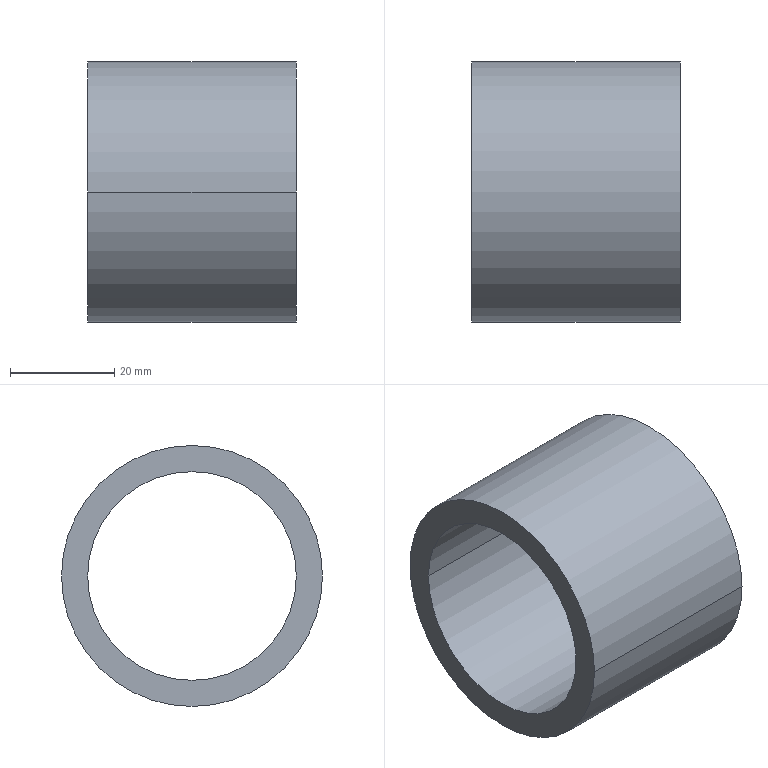Part | STEP file | P-0082107 | 1 solid | 6 faces | box 40 x 50 x 50 mm | volume 28274 mm3 | cylinder 4 | plane 2 | commonest cylinder face diameters 40 x2 50 x2
STEP:
#1=CARTESIAN_POINT('',(0.,0.,0.));
#2=DIRECTION('',(0.,0.,1.));
#3=DIRECTION('',(1.,0.,0.));
#4=AXIS2_PLACEMENT_3D('',#1,#2,#3);
#5=CARTESIAN_POINT('',(-30.,20.,0.));
#6=VERTEX_POINT('',#5);
#7=CARTESIAN_POINT('',(-30.,-20.,0.));
#8=VERTEX_POINT('',#7);
#9=CARTESIAN_POINT('',(-30.,0.,0.));
#10=DIRECTION('',(-1.,0.,0.));
#11=DIRECTION('',(0.,1.,0.));
#12=AXIS2_PLACEMENT_3D('',#9,#10,#11);
#13=CIRCLE('',#12,20.);
#14=CARTESIAN_POINT('',(-30.,0.,0.));
#15=DIRECTION('',(1.,0.,0.));
#16=DIRECTION('',(0.,1.,0.));
#17=AXIS2_PLACEMENT_3D('',#14,#15,#16);
#18=PLANE('',#17);
#19=CARTESIAN_POINT('',(20.,0.));
#20=CARTESIAN_POINT('',(20.,-34.641));
#21=CARTESIAN_POINT('',(-10.,-17.321));
#22=CARTESIAN_POINT('',(-40.,0.));
#23=CARTESIAN_POINT('',(-10.,17.321));
#24=CARTESIAN_POINT('',(20.,34.641));
#25=CARTESIAN_POINT('',(20.,0.));
#26=(BOUNDED_CURVE()B_SPLINE_CURVE(2,(#19,#20,#21,#22,#23,#24,#25),.UNSPECIFIED.,.T.,.F.)B_SPLINE_CURVE_WITH_KNOTS((1,2,2,2,2,1),(-2.094,0.,2.094,4.189,6.283,8.378),.UNSPECIFIED.)CURVE()GEOMETRIC_REPRESENTATION_ITEM()RATIONAL_B_SPLINE_CURVE((1.,0.5,1.,0.5,1.,0.5,1.))REPRESENTATION_ITEM(''));
#27=(GEOMETRIC_REPRESENTATION_CONTEXT(2)PARAMETRIC_REPRESENTATION_CONTEXT()REPRESENTATION_CONTEXT('',''));
#28=DEFINITIONAL_REPRESENTATION('',(#26),#27);
#29=PCURVE('',#18,#28);
#30=CARTESIAN_POINT('',(-30.,0.,0.));
#31=DIRECTION('',(1.,0.,0.));
#32=DIRECTION('',(0.,1.,0.));
#33=AXIS2_PLACEMENT_3D('',#30,#31,#32);
#34=CYLINDRICAL_SURFACE('',#33,20.);
#35=CARTESIAN_POINT('',(6.283,0.));
#36=DIRECTION('',(-1.,0.));
#37=VECTOR('',#36,1.);
#38=LINE('',#35,#37);
#39=(GEOMETRIC_REPRESENTATION_CONTEXT(2)PARAMETRIC_REPRESENTATION_CONTEXT()REPRESENTATION_CONTEXT('',''));
#40=DEFINITIONAL_REPRESENTATION('',(#38),#39);
#41=PCURVE('',#34,#40);
#42=SURFACE_CURVE('',#13,(#29,#41),.PCURVE_S1.);
#43=EDGE_CURVE('',#6,#8,#42,.T.);
#44=ORIENTED_EDGE('',*,*,#43,.F.);
#45=CARTESIAN_POINT('',(-30.,0.,0.));
#46=DIRECTION('',(-1.,0.,0.));
#47=DIRECTION('',(0.,1.,0.));
#48=AXIS2_PLACEMENT_3D('',#45,#46,#47);
#49=CIRCLE('',#48,20.);
#50=CARTESIAN_POINT('',(20.,0.));
#51=CARTESIAN_POINT('',(20.,-34.641));
#52=CARTESIAN_POINT('',(-10.,-17.321));
#53=CARTESIAN_POINT('',(-40.,0.));
#54=CARTESIAN_POINT('',(-10.,17.321));
#55=CARTESIAN_POINT('',(20.,34.641));
#56=CARTESIAN_POINT('',(20.,0.));
#57=(BOUNDED_CURVE()B_SPLINE_CURVE(2,(#50,#51,#52,#53,#54,#55,#56),.UNSPECIFIED.,.T.,.F.)B_SPLINE_CURVE_WITH_KNOTS((1,2,2,2,2,1),(-2.094,0.,2.094,4.189,6.283,8.378),.UNSPECIFIED.)CURVE()GEOMETRIC_REPRESENTATION_ITEM()RATIONAL_B_SPLINE_CURVE((1.,0.5,1.,0.5,1.,0.5,1.))REPRESENTATION_ITEM(''));
#58=(GEOMETRIC_REPRESENTATION_CONTEXT(2)PARAMETRIC_REPRESENTATION_CONTEXT()REPRESENTATION_CONTEXT('',''));
#59=DEFINITIONAL_REPRESENTATION('',(#57),#58);
#60=PCURVE('',#18,#59);
#61=CARTESIAN_POINT('',(-30.,0.,0.));
#62=DIRECTION('',(1.,0.,0.));
#63=DIRECTION('',(0.,1.,0.));
#64=AXIS2_PLACEMENT_3D('',#61,#62,#63);
#65=CYLINDRICAL_SURFACE('',#64,20.);
#66=CARTESIAN_POINT('',(6.283,0.));
#67=DIRECTION('',(-1.,0.));
#68=VECTOR('',#67,1.);
#69=LINE('',#66,#68);
#70=(GEOMETRIC_REPRESENTATION_CONTEXT(2)PARAMETRIC_REPRESENTATION_CONTEXT()REPRESENTATION_CONTEXT('',''));
#71=DEFINITIONAL_REPRESENTATION('',(#69),#70);
#72=PCURVE('',#65,#71);
#73=SURFACE_CURVE('',#49,(#60,#72),.PCURVE_S1.);
#74=EDGE_CURVE('',#8,#6,#73,.T.);
#75=ORIENTED_EDGE('',*,*,#74,.F.);
#76=EDGE_LOOP('',(#44,#75));
#77=FACE_BOUND('',#76,.T.);
#78=CARTESIAN_POINT('',(-30.,25.,0.));
#79=VERTEX_POINT('',#78);
#80=CARTESIAN_POINT('',(-30.,-25.,0.));
#81=VERTEX_POINT('',#80);
#82=CARTESIAN_POINT('',(-30.,0.,0.));
#83=DIRECTION('',(1.,0.,0.));
#84=DIRECTION('',(0.,1.,0.));
#85=AXIS2_PLACEMENT_3D('',#82,#83,#84);
#86=CIRCLE('',#85,25.);
#87=CARTESIAN_POINT('',(0.,0.));
#88=DIRECTION('',(1.,0.));
#89=AXIS2_PLACEMENT_2D('',#87,#88);
#90=CIRCLE('',#89,25.);
#91=(GEOMETRIC_REPRESENTATION_CONTEXT(2)PARAMETRIC_REPRESENTATION_CONTEXT()REPRESENTATION_CONTEXT('',''));
#92=DEFINITIONAL_REPRESENTATION('',(#90),#91);
#93=PCURVE('',#18,#92);
#94=CARTESIAN_POINT('',(-30.,0.,0.));
#95=DIRECTION('',(1.,0.,0.));
#96=DIRECTION('',(0.,1.,0.));
#97=AXIS2_PLACEMENT_3D('',#94,#95,#96);
#98=CYLINDRICAL_SURFACE('',#97,25.);
#99=CARTESIAN_POINT('',(0.,0.));
#100=DIRECTION('',(1.,0.));
#101=VECTOR('',#100,1.);
#102=LINE('',#99,#101);
#103=(GEOMETRIC_REPRESENTATION_CONTEXT(2)PARAMETRIC_REPRESENTATION_CONTEXT()REPRESENTATION_CONTEXT('',''));
#104=DEFINITIONAL_REPRESENTATION('',(#102),#103);
#105=PCURVE('',#98,#104);
#106=SURFACE_CURVE('',#86,(#93,#105),.PCURVE_S1.);
#107=EDGE_CURVE('',#79,#81,#106,.T.);
#108=ORIENTED_EDGE('',*,*,#107,.F.);
#109=CARTESIAN_POINT('',(-30.,0.,0.));
#110=DIRECTION('',(1.,0.,0.));
#111=DIRECTION('',(0.,1.,0.));
#112=AXIS2_PLACEMENT_3D('',#109,#110,#111);
#113=CIRCLE('',#112,25.);
#114=CARTESIAN_POINT('',(0.,0.));
#115=DIRECTION('',(1.,0.));
#116=AXIS2_PLACEMENT_2D('',#114,#115);
#117=CIRCLE('',#116,25.);
#118=(GEOMETRIC_REPRESENTATION_CONTEXT(2)PARAMETRIC_REPRESENTATION_CONTEXT()REPRESENTATION_CONTEXT('',''));
#119=DEFINITIONAL_REPRESENTATION('',(#117),#118);
#120=PCURVE('',#18,#119);
#121=CARTESIAN_POINT('',(-30.,0.,0.));
#122=DIRECTION('',(1.,0.,0.));
#123=DIRECTION('',(0.,1.,0.));
#124=AXIS2_PLACEMENT_3D('',#121,#122,#123);
#125=CYLINDRICAL_SURFACE('',#124,25.);
#126=CARTESIAN_POINT('',(0.,0.));
#127=DIRECTION('',(1.,0.));
#128=VECTOR('',#127,1.);
#129=LINE('',#126,#128);
#130=(GEOMETRIC_REPRESENTATION_CONTEXT(2)PARAMETRIC_REPRESENTATION_CONTEXT()REPRESENTATION_CONTEXT('',''));
#131=DEFINITIONAL_REPRESENTATION('',(#129),#130);
#132=PCURVE('',#125,#131);
#133=SURFACE_CURVE('',#113,(#120,#132),.PCURVE_S1.);
#134=EDGE_CURVE('',#81,#79,#133,.T.);
#135=ORIENTED_EDGE('',*,*,#134,.F.);
#136=EDGE_LOOP('',(#108,#135));
#137=FACE_BOUND('',#136,.T.);
#138=ADVANCED_FACE('',(#77,#137),#18,.F.);
#139=CARTESIAN_POINT('',(10.,20.,0.));
#140=VERTEX_POINT('',#139);
#141=CARTESIAN_POINT('',(10.,-20.,0.));
#142=VERTEX_POINT('',#141);
#143=CARTESIAN_POINT('',(10.,0.,0.));
#144=DIRECTION('',(1.,0.,0.));
#145=DIRECTION('',(0.,1.,0.));
#146=AXIS2_PLACEMENT_3D('',#143,#144,#145);
#147=CIRCLE('',#146,20.);
#148=CARTESIAN_POINT('',(10.,0.,0.));
#149=DIRECTION('',(1.,0.,0.));
#150=DIRECTION('',(0.,1.,0.));
#151=AXIS2_PLACEMENT_3D('',#148,#149,#150);
#152=PLANE('',#151);
#153=CARTESIAN_POINT('',(0.,0.));
#154=DIRECTION('',(1.,0.));
#155=AXIS2_PLACEMENT_2D('',#153,#154);
#156=CIRCLE('',#155,20.);
#157=(GEOMETRIC_REPRESENTATION_CONTEXT(2)PARAMETRIC_REPRESENTATION_CONTEXT()REPRESENTATION_CONTEXT('',''));
#158=DEFINITIONAL_REPRESENTATION('',(#156),#157);
#159=PCURVE('',#152,#158);
#160=CARTESIAN_POINT('',(0.,40.));
#161=DIRECTION('',(1.,0.));
#162=VECTOR('',#161,1.);
#163=LINE('',#160,#162);
#164=(GEOMETRIC_REPRESENTATION_CONTEXT(2)PARAMETRIC_REPRESENTATION_CONTEXT()REPRESENTATION_CONTEXT('',''));
#165=DEFINITIONAL_REPRESENTATION('',(#163),#164);
#166=PCURVE('',#65,#165);
#167=SURFACE_CURVE('',#147,(#159,#166),.PCURVE_S1.);
#168=EDGE_CURVE('',#140,#142,#167,.T.);
#169=ORIENTED_EDGE('',*,*,#168,.F.);
#170=CARTESIAN_POINT('',(10.,0.,0.));
#171=DIRECTION('',(1.,0.,0.));
#172=DIRECTION('',(0.,1.,0.));
#173=AXIS2_PLACEMENT_3D('',#170,#171,#172);
#174=CIRCLE('',#173,20.);
#175=CARTESIAN_POINT('',(0.,0.));
#176=DIRECTION('',(1.,0.));
#177=AXIS2_PLACEMENT_2D('',#175,#176);
#178=CIRCLE('',#177,20.);
#179=(GEOMETRIC_REPRESENTATION_CONTEXT(2)PARAMETRIC_REPRESENTATION_CONTEXT()REPRESENTATION_CONTEXT('',''));
#180=DEFINITIONAL_REPRESENTATION('',(#178),#179);
#181=PCURVE('',#152,#180);
#182=CARTESIAN_POINT('',(0.,40.));
#183=DIRECTION('',(1.,0.));
#184=VECTOR('',#183,1.);
#185=LINE('',#182,#184);
#186=(GEOMETRIC_REPRESENTATION_CONTEXT(2)PARAMETRIC_REPRESENTATION_CONTEXT()REPRESENTATION_CONTEXT('',''));
#187=DEFINITIONAL_REPRESENTATION('',(#185),#186);
#188=PCURVE('',#34,#187);
#189=SURFACE_CURVE('',#174,(#181,#188),.PCURVE_S1.);
#190=EDGE_CURVE('',#142,#140,#189,.T.);
#191=ORIENTED_EDGE('',*,*,#190,.F.);
#192=EDGE_LOOP('',(#169,#191));
#193=FACE_BOUND('',#192,.T.);
#194=CARTESIAN_POINT('',(10.,25.,0.));
#195=VERTEX_POINT('',#194);
#196=CARTESIAN_POINT('',(10.,-25.,0.));
#197=VERTEX_POINT('',#196);
#198=CARTESIAN_POINT('',(10.,0.,0.));
#199=DIRECTION('',(-1.,0.,0.));
#200=DIRECTION('',(0.,1.,0.));
#201=AXIS2_PLACEMENT_3D('',#198,#199,#200);
#202=CIRCLE('',#201,25.);
#203=CARTESIAN_POINT('',(25.,0.));
#204=CARTESIAN_POINT('',(25.,-43.301));
#205=CARTESIAN_POINT('',(-12.5,-21.651));
#206=CARTESIAN_POINT('',(-50.,0.));
#207=CARTESIAN_POINT('',(-12.5,21.651));
#208=CARTESIAN_POINT('',(25.,43.301));
#209=CARTESIAN_POINT('',(25.,0.));
#210=(BOUNDED_CURVE()B_SPLINE_CURVE(2,(#203,#204,#205,#206,#207,#208,#209),.UNSPECIFIED.,.T.,.F.)B_SPLINE_CURVE_WITH_KNOTS((1,2,2,2,2,1),(-2.094,0.,2.094,4.189,6.283,8.378),.UNSPECIFIED.)CURVE()GEOMETRIC_REPRESENTATION_ITEM()RATIONAL_B_SPLINE_CURVE((1.,0.5,1.,0.5,1.,0.5,1.))REPRESENTATION_ITEM(''));
#211=(GEOMETRIC_REPRESENTATION_CONTEXT(2)PARAMETRIC_REPRESENTATION_CONTEXT()REPRESENTATION_CONTEXT('',''));
#212=DEFINITIONAL_REPRESENTATION('',(#210),#211);
#213=PCURVE('',#152,#212);
#214=CARTESIAN_POINT('',(6.283,40.));
#215=DIRECTION('',(-1.,0.));
#216=VECTOR('',#215,1.);
#217=LINE('',#214,#216);
#218=(GEOMETRIC_REPRESENTATION_CONTEXT(2)PARAMETRIC_REPRESENTATION_CONTEXT()REPRESENTATION_CONTEXT('',''));
#219=DEFINITIONAL_REPRESENTATION('',(#217),#218);
#220=PCURVE('',#125,#219);
#221=SURFACE_CURVE('',#202,(#213,#220),.PCURVE_S1.);
#222=EDGE_CURVE('',#195,#197,#221,.T.);
#223=ORIENTED_EDGE('',*,*,#222,.F.);
#224=CARTESIAN_POINT('',(10.,0.,0.));
#225=DIRECTION('',(-1.,0.,0.));
#226=DIRECTION('',(0.,1.,0.));
#227=AXIS2_PLACEMENT_3D('',#224,#225,#226);
#228=CIRCLE('',#227,25.);
#229=CARTESIAN_POINT('',(25.,0.));
#230=CARTESIAN_POINT('',(25.,-43.301));
#231=CARTESIAN_POINT('',(-12.5,-21.651));
#232=CARTESIAN_POINT('',(-50.,0.));
#233=CARTESIAN_POINT('',(-12.5,21.651));
#234=CARTESIAN_POINT('',(25.,43.301));
#235=CARTESIAN_POINT('',(25.,0.));
#236=(BOUNDED_CURVE()B_SPLINE_CURVE(2,(#229,#230,#231,#232,#233,#234,#235),.UNSPECIFIED.,.T.,.F.)B_SPLINE_CURVE_WITH_KNOTS((1,2,2,2,2,1),(-2.094,0.,2.094,4.189,6.283,8.378),.UNSPECIFIED.)CURVE()GEOMETRIC_REPRESENTATION_ITEM()RATIONAL_B_SPLINE_CURVE((1.,0.5,1.,0.5,1.,0.5,1.))REPRESENTATION_ITEM(''));
#237=(GEOMETRIC_REPRESENTATION_CONTEXT(2)PARAMETRIC_REPRESENTATION_CONTEXT()REPRESENTATION_CONTEXT('',''));
#238=DEFINITIONAL_REPRESENTATION('',(#236),#237);
#239=PCURVE('',#152,#238);
#240=CARTESIAN_POINT('',(6.283,40.));
#241=DIRECTION('',(-1.,0.));
#242=VECTOR('',#241,1.);
#243=LINE('',#240,#242);
#244=(GEOMETRIC_REPRESENTATION_CONTEXT(2)PARAMETRIC_REPRESENTATION_CONTEXT()REPRESENTATION_CONTEXT('',''));
#245=DEFINITIONAL_REPRESENTATION('',(#243),#244);
#246=PCURVE('',#98,#245);
#247=SURFACE_CURVE('',#228,(#239,#246),.PCURVE_S1.);
#248=EDGE_CURVE('',#197,#195,#247,.T.);
#249=ORIENTED_EDGE('',*,*,#248,.F.);
#250=EDGE_LOOP('',(#223,#249));
#251=FACE_BOUND('',#250,.T.);
#252=ADVANCED_FACE('',(#193,#251),#152,.T.);
#253=ORIENTED_EDGE('',*,*,#190,.F.);
#254=CARTESIAN_POINT('',(10.,-20.,0.));
#255=DIRECTION('',(-1.,0.,0.));
#256=VECTOR('',#255,1.);
#257=LINE('',#254,#256);
#258=CARTESIAN_POINT('',(3.142,40.));
#259=DIRECTION('',(0.,-1.));
#260=VECTOR('',#259,1.);
#261=LINE('',#258,#260);
#262=(GEOMETRIC_REPRESENTATION_CONTEXT(2)PARAMETRIC_REPRESENTATION_CONTEXT()REPRESENTATION_CONTEXT('',''));
#263=DEFINITIONAL_REPRESENTATION('',(#261),#262);
#264=PCURVE('',#34,#263);
#265=CARTESIAN_POINT('',(3.142,40.));
#266=DIRECTION('',(0.,-1.));
#267=VECTOR('',#266,1.);
#268=LINE('',#265,#267);
#269=(GEOMETRIC_REPRESENTATION_CONTEXT(2)PARAMETRIC_REPRESENTATION_CONTEXT()REPRESENTATION_CONTEXT('',''));
#270=DEFINITIONAL_REPRESENTATION('',(#268),#269);
#271=PCURVE('',#65,#270);
#272=SURFACE_CURVE('',#257,(#264,#271),.PCURVE_S1.);
#273=EDGE_CURVE('',#142,#8,#272,.T.);
#274=ORIENTED_EDGE('',*,*,#273,.T.);
#275=ORIENTED_EDGE('',*,*,#43,.F.);
#276=CARTESIAN_POINT('',(10.,20.,0.));
#277=DIRECTION('',(-1.,0.,0.));
#278=VECTOR('',#277,1.);
#279=LINE('',#276,#278);
#280=CARTESIAN_POINT('',(6.283,40.));
#281=DIRECTION('',(0.,-1.));
#282=VECTOR('',#281,1.);
#283=LINE('',#280,#282);
#284=(GEOMETRIC_REPRESENTATION_CONTEXT(2)PARAMETRIC_REPRESENTATION_CONTEXT()REPRESENTATION_CONTEXT('',''));
#285=DEFINITIONAL_REPRESENTATION('',(#283),#284);
#286=PCURVE('',#34,#285);
#287=CARTESIAN_POINT('',(0.,40.));
#288=DIRECTION('',(0.,-1.));
#289=VECTOR('',#288,1.);
#290=LINE('',#287,#289);
#291=(GEOMETRIC_REPRESENTATION_CONTEXT(2)PARAMETRIC_REPRESENTATION_CONTEXT()REPRESENTATION_CONTEXT('',''));
#292=DEFINITIONAL_REPRESENTATION('',(#290),#291);
#293=PCURVE('',#65,#292);
#294=SURFACE_CURVE('',#279,(#286,#293),.PCURVE_S1.);
#295=EDGE_CURVE('',#140,#6,#294,.T.);
#296=ORIENTED_EDGE('',*,*,#295,.F.);
#297=EDGE_LOOP('',(#253,#274,#275,#296));
#298=FACE_BOUND('',#297,.F.);
#299=ADVANCED_FACE('',(#298),#34,.F.);
#300=CARTESIAN_POINT('',(10.,25.,0.));
#301=DIRECTION('',(-1.,0.,0.));
#302=VECTOR('',#301,1.);
#303=LINE('',#300,#302);
#304=CARTESIAN_POINT('',(0.,40.));
#305=DIRECTION('',(0.,-1.));
#306=VECTOR('',#305,1.);
#307=LINE('',#304,#306);
#308=(GEOMETRIC_REPRESENTATION_CONTEXT(2)PARAMETRIC_REPRESENTATION_CONTEXT()REPRESENTATION_CONTEXT('',''));
#309=DEFINITIONAL_REPRESENTATION('',(#307),#308);
#310=PCURVE('',#98,#309);
#311=CARTESIAN_POINT('',(6.283,40.));
#312=DIRECTION('',(0.,-1.));
#313=VECTOR('',#312,1.);
#314=LINE('',#311,#313);
#315=(GEOMETRIC_REPRESENTATION_CONTEXT(2)PARAMETRIC_REPRESENTATION_CONTEXT()REPRESENTATION_CONTEXT('',''));
#316=DEFINITIONAL_REPRESENTATION('',(#314),#315);
#317=PCURVE('',#125,#316);
#318=SURFACE_CURVE('',#303,(#310,#317),.PCURVE_S1.);
#319=EDGE_CURVE('',#195,#79,#318,.T.);
#320=ORIENTED_EDGE('',*,*,#319,.T.);
#321=ORIENTED_EDGE('',*,*,#107,.T.);
#322=CARTESIAN_POINT('',(10.,-25.,0.));
#323=DIRECTION('',(-1.,0.,0.));
#324=VECTOR('',#323,1.);
#325=LINE('',#322,#324);
#326=CARTESIAN_POINT('',(3.142,40.));
#327=DIRECTION('',(0.,-1.));
#328=VECTOR('',#327,1.);
#329=LINE('',#326,#328);
#330=(GEOMETRIC_REPRESENTATION_CONTEXT(2)PARAMETRIC_REPRESENTATION_CONTEXT()REPRESENTATION_CONTEXT('',''));
#331=DEFINITIONAL_REPRESENTATION('',(#329),#330);
#332=PCURVE('',#98,#331);
#333=CARTESIAN_POINT('',(3.142,40.));
#334=DIRECTION('',(0.,-1.));
#335=VECTOR('',#334,1.);
#336=LINE('',#333,#335);
#337=(GEOMETRIC_REPRESENTATION_CONTEXT(2)PARAMETRIC_REPRESENTATION_CONTEXT()REPRESENTATION_CONTEXT('',''));
#338=DEFINITIONAL_REPRESENTATION('',(#336),#337);
#339=PCURVE('',#125,#338);
#340=SURFACE_CURVE('',#325,(#332,#339),.PCURVE_S1.);
#341=EDGE_CURVE('',#197,#81,#340,.T.);
#342=ORIENTED_EDGE('',*,*,#341,.F.);
#343=ORIENTED_EDGE('',*,*,#248,.T.);
#344=EDGE_LOOP('',(#320,#321,#342,#343));
#345=FACE_BOUND('',#344,.T.);
#346=ADVANCED_FACE('',(#345),#98,.T.);
#347=ORIENTED_EDGE('',*,*,#319,.F.);
#348=ORIENTED_EDGE('',*,*,#222,.T.);
#349=ORIENTED_EDGE('',*,*,#341,.T.);
#350=ORIENTED_EDGE('',*,*,#134,.T.);
#351=EDGE_LOOP('',(#347,#348,#349,#350));
#352=FACE_BOUND('',#351,.T.);
#353=ADVANCED_FACE('',(#352),#125,.T.);
#354=ORIENTED_EDGE('',*,*,#74,.F.);
#355=ORIENTED_EDGE('',*,*,#273,.F.);
#356=ORIENTED_EDGE('',*,*,#168,.F.);
#357=ORIENTED_EDGE('',*,*,#295,.T.);
#358=EDGE_LOOP('',(#354,#355,#356,#357));
#359=FACE_BOUND('',#358,.F.);
#360=ADVANCED_FACE('',(#359),#65,.F.);
#361=CLOSED_SHELL('',(#138,#252,#299,#346,#353,#360));
#362=MANIFOLD_SOLID_BREP('',#361);
#363=(LENGTH_UNIT()NAMED_UNIT(*)SI_UNIT(.MILLI.,.METRE.));
#364=UNCERTAINTY_MEASURE_WITH_UNIT(LENGTH_MEASURE(0.0000001),#363,'','');
#365=(NAMED_UNIT(*)PLANE_ANGLE_UNIT()SI_UNIT($,.RADIAN.));
#366=(NAMED_UNIT(*)SI_UNIT($,.STERADIAN.)SOLID_ANGLE_UNIT());
#367=(GEOMETRIC_REPRESENTATION_CONTEXT(3)GLOBAL_UNCERTAINTY_ASSIGNED_CONTEXT((#364))GLOBAL_UNIT_ASSIGNED_CONTEXT((#363,#365,#366))REPRESENTATION_CONTEXT('',''));
#368=ADVANCED_BREP_SHAPE_REPRESENTATION('',(#4,#362),#367);